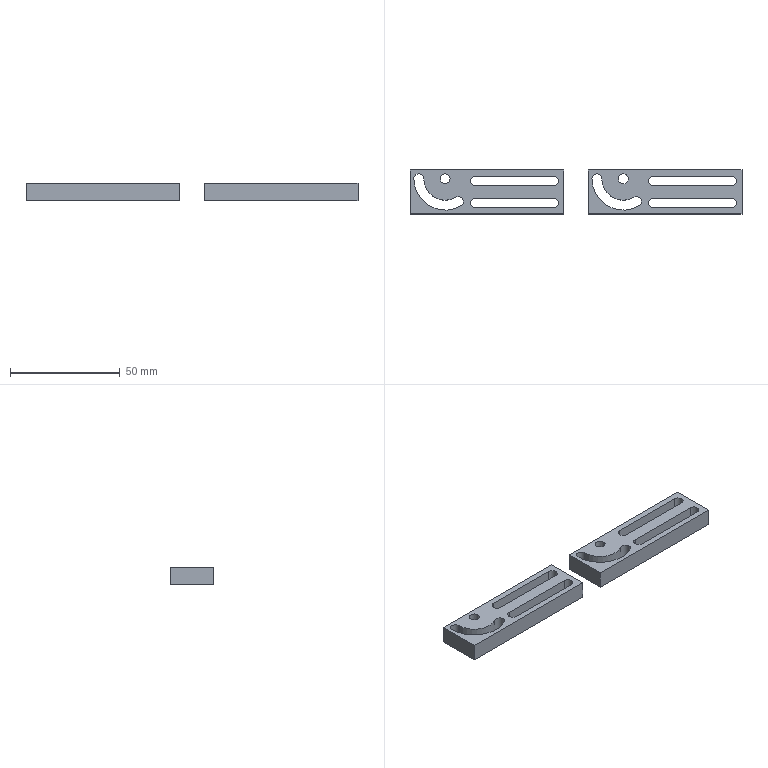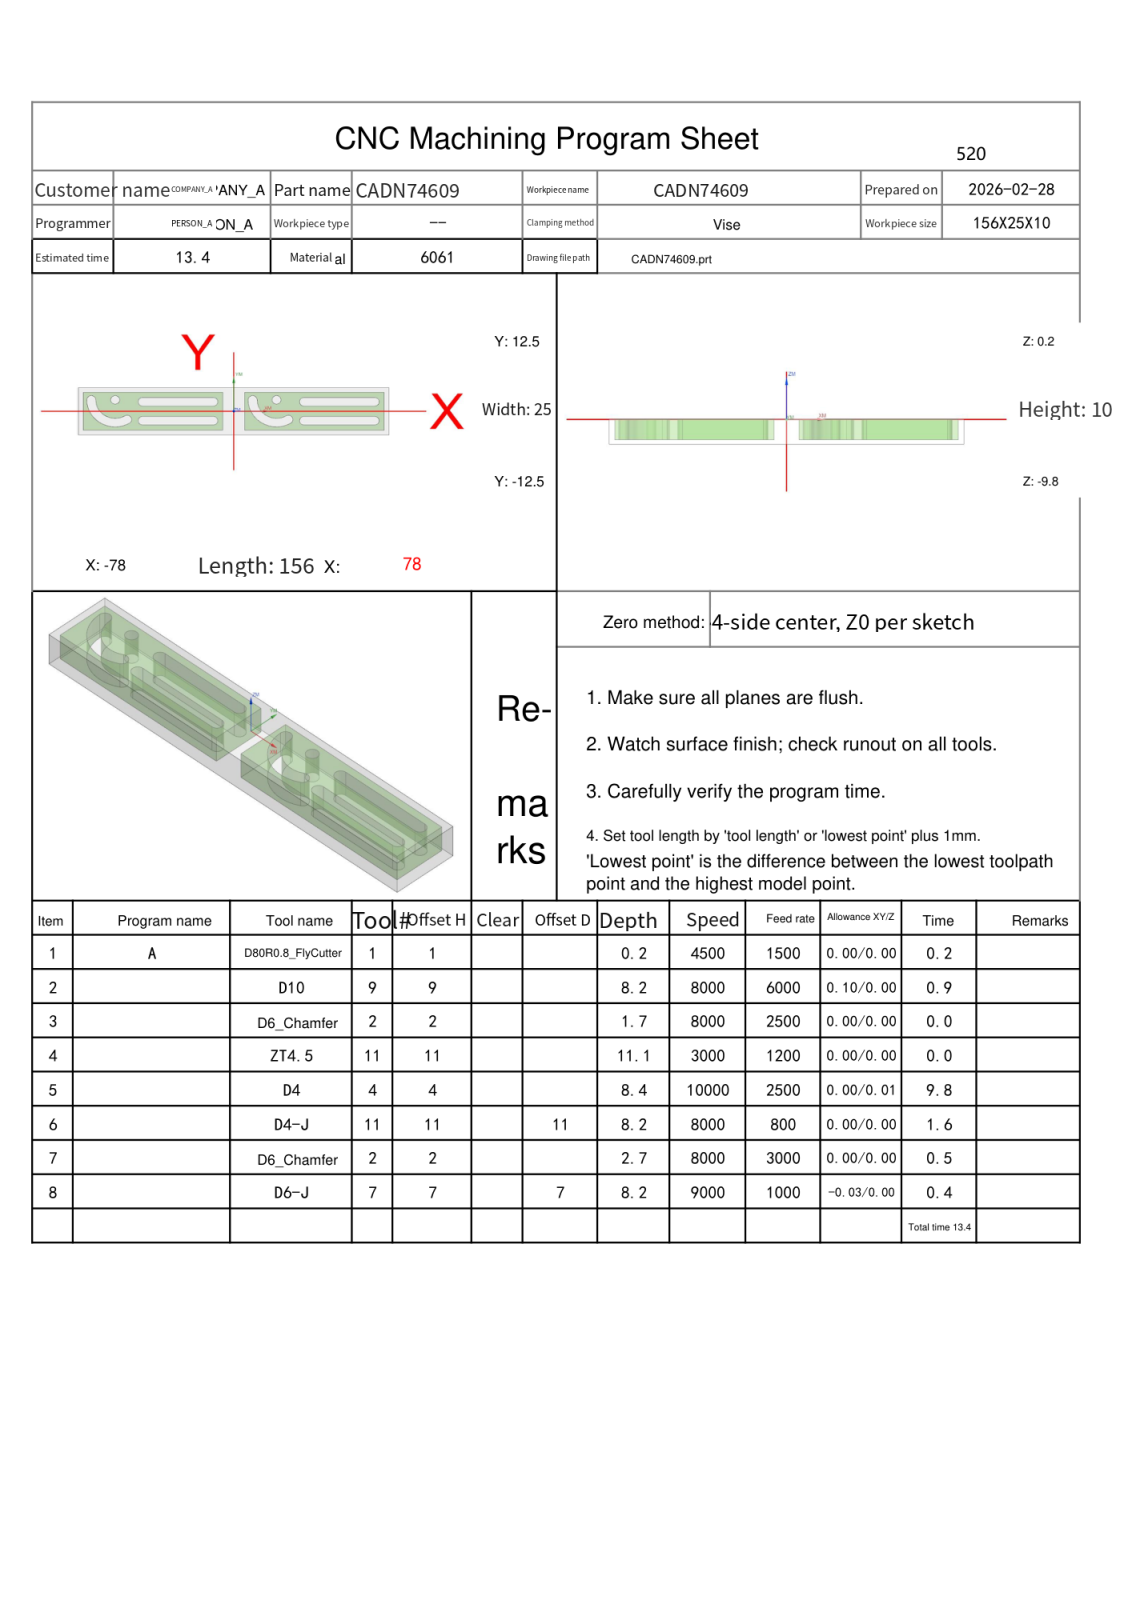NC program | NX | posted by the shop | part box 151 x 20 x 8 mm
Lines 1 to 275 of 3746:
%
O0001
(Machine time: 14.93 MIN)
(===Total Tool:6===)
(T1=D80R0.8-FlyCutter D=80.  R=0.8  D-  H01 Z=0.    )
(T9=D10     D=10.  R=0.   D-  H09 Z=-8.   )
(T2=D6_Chamfer   D=6.   R=0.   D-  H02 Z=-2.55 )
(T11=ZT4.5  D=4.5  DR_a=118 D-  H11 Z=-10.85)
(T4=D4      D=4.   R=0.   D-  H04 Z=-8.2  )
(T7=D6-J    D=6.   R=0.   D7  H07 Z=-8.   )
G80 G90 G17 G49 G40
G91 G28 Z0
M01
N1 T01 M06
(D80R0.8-FlyCutter  D=80. R=0.8 H=01 ce=0.00 di=0.00)
G00 G90 G54 X-120.5 Y0.0 M03 S4500
G43 H01 Z50.
M08
Z2.
G01 Z0.0 F1500.
X-115.5
X115.5
X120.5
Z2.
G00 Z50.
G91 G28 Z0.0
M05
M09
G91 G28 Z0.0
M01
N2 T09 M06
(D10  D=10. R=0. H=09 ce=0.10 di=0.00)
G00 G90 G54 X-40.5 Y-15.1 M03 S8000
G43 H09 Z50.
M08
Z.5
G01 X-75.5 Z.372 F6000.
G02 X-80.6 Y-10. Z.343 I0.0 J5.1
G01 Y10. Z.27
G02 X-75.5 Y15.1 Z.241 I5.1 J0.0
G01 X-5.5 Z-.014
G02 X-.4 Y10. Z-.043 I0.0 J-5.1
G01 Y-10. Z-.116
G02 X-5.5 Y-15.1 Z-.145 I-5.1 J0.0
G01 X-75.5 Z-.4
G02 X-80.6 Y-10. Z-.429 I0.0 J5.1
G01 Y10. Z-.502
G02 X-75.5 Y15.1 Z-.532 I5.1 J0.0
G01 X-5.5 Z-.787
G02 X-.4 Y10. Z-.816 I0.0 J-5.1
G01 Y-10. Z-.889
G02 X-5.5 Y-15.1 Z-.918 I-5.1 J0.0
G01 X-75.5 Z-1.173
G02 X-80.6 Y-10. Z-1.202 I0.0 J5.1
G01 Y10. Z-1.275
G02 X-75.5 Y15.1 Z-1.304 I5.1 J0.0
G01 X-5.5 Z-1.559
G02 X-.4 Y10. Z-1.589 I0.0 J-5.1
G01 Y-10. Z-1.661
G02 X-5.5 Y-15.1 Z-1.691 I-5.1 J0.0
G01 X-75.5 Z-1.946
G02 X-80.6 Y-10. Z-1.975 I0.0 J5.1
G01 Y10. Z-2.048
G02 X-75.5 Y15.1 Z-2.077 I5.1 J0.0
G01 X-5.5 Z-2.332
G02 X-.4 Y10. Z-2.361 I0.0 J-5.1
G01 Y-10. Z-2.434
G02 X-5.5 Y-15.1 Z-2.463 I-5.1 J0.0
G01 X-75.5 Z-2.718
G02 X-80.6 Y-10. Z-2.748 I0.0 J5.1
G01 Y10. Z-2.821
G02 X-75.5 Y15.1 Z-2.85 I5.1 J0.0
G01 X-5.5 Z-3.105
G02 X-.4 Y10. Z-3.134 I0.0 J-5.1
G01 Y-10. Z-3.207
G02 X-5.5 Y-15.1 Z-3.236 I-5.1 J0.0
G01 X-75.5 Z-3.491
G02 X-80.6 Y-10. Z-3.52 I0.0 J5.1
G01 Y10. Z-3.593
G02 X-75.5 Y15.1 Z-3.622 I5.1 J0.0
G01 X-5.5 Z-3.878
G02 X-.4 Y10. Z-3.907 I0.0 J-5.1
G01 Y-10. Z-3.98
G02 X-5.5 Y-15.1 Z-4.009 I-5.1 J0.0
G01 X-75.5 Z-4.264
G02 X-80.6 Y-10. Z-4.293 I0.0 J5.1
G01 Y10. Z-4.366
G02 X-75.5 Y15.1 Z-4.395 I5.1 J0.0
G01 X-5.5 Z-4.65
G02 X-.4 Y10. Z-4.679 I0.0 J-5.1
G01 Y-10. Z-4.752
G02 X-5.5 Y-15.1 Z-4.782 I-5.1 J0.0
G01 X-75.5 Z-5.037
G02 X-80.6 Y-10. Z-5.066 I0.0 J5.1
G01 Y10. Z-5.139
G02 X-75.5 Y15.1 Z-5.168 I5.1 J0.0
G01 X-5.5 Z-5.423
G02 X-.4 Y10. Z-5.452 I0.0 J-5.1
G01 Y-10. Z-5.525
G02 X-5.5 Y-15.1 Z-5.554 I-5.1 J0.0
G01 X-75.5 Z-5.809
G02 X-80.6 Y-10. Z-5.839 I0.0 J5.1
G01 Y10. Z-5.911
G02 X-75.5 Y15.1 Z-5.941 I5.1 J0.0
G01 X-5.5 Z-6.196
G02 X-.4 Y10. Z-6.225 I0.0 J-5.1
G01 Y-10. Z-6.298
G02 X-5.5 Y-15.1 Z-6.327 I-5.1 J0.0
G01 X-75.5 Z-6.582
G02 X-80.6 Y-10. Z-6.611 I0.0 J5.1
G01 Y10. Z-6.684
G02 X-75.5 Y15.1 Z-6.713 I5.1 J0.0
G01 X-5.5 Z-6.968
G02 X-.4 Y10. Z-6.998 I0.0 J-5.1
G01 Y-10. Z-7.071
G02 X-5.5 Y-15.1 Z-7.1 I-5.1 J0.0
G01 X-75.5 Z-7.355
G02 X-80.6 Y-10. Z-7.384 I0.0 J5.1
G01 Y10. Z-7.457
G02 X-75.5 Y15.1 Z-7.486 I5.1 J0.0
G01 X-5.5 Z-7.741
G02 X-.4 Y10. Z-7.77 I0.0 J-5.1
G01 Y-10. Z-7.843
G02 X-5.5 Y-15.1 Z-7.872 I-5.1 J0.0
G01 X-40.5 Z-8.
X-75.5
G02 X-80.6 Y-10. I0.0 J5.1
G01 Y10.
G02 X-75.5 Y15.1 I5.1 J0.0
G01 X-5.5
G02 X-.4 Y10. I0.0 J-5.1
G01 Y-10.
G02 X-5.5 Y-15.1 I-5.1 J0.0
G01 X-40.5
X-41.
Z-7.
G00 Z50.
X40.5
Z.5
G01 X5.5 Z.372
G02 X.4 Y-10. Z.343 I0.0 J5.1
G01 Y10. Z.27
G02 X5.5 Y15.1 Z.241 I5.1 J0.0
G01 X75.5 Z-.014
G02 X80.6 Y10. Z-.043 I0.0 J-5.1
G01 Y-10. Z-.116
G02 X75.5 Y-15.1 Z-.145 I-5.1 J0.0
G01 X5.5 Z-.4
G02 X.4 Y-10. Z-.429 I0.0 J5.1
G01 Y10. Z-.502
G02 X5.5 Y15.1 Z-.532 I5.1 J0.0
G01 X75.5 Z-.787
G02 X80.6 Y10. Z-.816 I0.0 J-5.1
G01 Y-10. Z-.889
G02 X75.5 Y-15.1 Z-.918 I-5.1 J0.0
G01 X5.5 Z-1.173
G02 X.4 Y-10. Z-1.202 I0.0 J5.1
G01 Y10. Z-1.275
G02 X5.5 Y15.1 Z-1.304 I5.1 J0.0
G01 X75.5 Z-1.559
G02 X80.6 Y10. Z-1.589 I0.0 J-5.1
G01 Y-10. Z-1.661
G02 X75.5 Y-15.1 Z-1.691 I-5.1 J0.0
G01 X5.5 Z-1.946
G02 X.4 Y-10. Z-1.975 I0.0 J5.1
G01 Y10. Z-2.048
G02 X5.5 Y15.1 Z-2.077 I5.1 J0.0
G01 X75.5 Z-2.332
G02 X80.6 Y10. Z-2.361 I0.0 J-5.1
G01 Y-10. Z-2.434
G02 X75.5 Y-15.1 Z-2.463 I-5.1 J0.0
G01 X5.5 Z-2.718
G02 X.4 Y-10. Z-2.748 I0.0 J5.1
G01 Y10. Z-2.821
G02 X5.5 Y15.1 Z-2.85 I5.1 J0.0
G01 X75.5 Z-3.105
G02 X80.6 Y10. Z-3.134 I0.0 J-5.1
G01 Y-10. Z-3.207
G02 X75.5 Y-15.1 Z-3.236 I-5.1 J0.0
G01 X5.5 Z-3.491
G02 X.4 Y-10. Z-3.52 I0.0 J5.1
G01 Y10. Z-3.593
G02 X5.5 Y15.1 Z-3.622 I5.1 J0.0
G01 X75.5 Z-3.878
G02 X80.6 Y10. Z-3.907 I0.0 J-5.1
G01 Y-10. Z-3.98
G02 X75.5 Y-15.1 Z-4.009 I-5.1 J0.0
G01 X5.5 Z-4.264
G02 X.4 Y-10. Z-4.293 I0.0 J5.1
G01 Y10. Z-4.366
G02 X5.5 Y15.1 Z-4.395 I5.1 J0.0
G01 X75.5 Z-4.65
G02 X80.6 Y10. Z-4.679 I0.0 J-5.1
G01 Y-10. Z-4.752
G02 X75.5 Y-15.1 Z-4.782 I-5.1 J0.0
G01 X5.5 Z-5.037
G02 X.4 Y-10. Z-5.066 I0.0 J5.1
G01 Y10. Z-5.139
G02 X5.5 Y15.1 Z-5.168 I5.1 J0.0
G01 X75.5 Z-5.423
G02 X80.6 Y10. Z-5.452 I0.0 J-5.1
G01 Y-10. Z-5.525
G02 X75.5 Y-15.1 Z-5.554 I-5.1 J0.0
G01 X5.5 Z-5.809
G02 X.4 Y-10. Z-5.839 I0.0 J5.1
G01 Y10. Z-5.911
G02 X5.5 Y15.1 Z-5.941 I5.1 J0.0
G01 X75.5 Z-6.196
G02 X80.6 Y10. Z-6.225 I0.0 J-5.1
G01 Y-10. Z-6.298
G02 X75.5 Y-15.1 Z-6.327 I-5.1 J0.0
G01 X5.5 Z-6.582
G02 X.4 Y-10. Z-6.611 I0.0 J5.1
G01 Y10. Z-6.684
G02 X5.5 Y15.1 Z-6.713 I5.1 J0.0
G01 X75.5 Z-6.968
G02 X80.6 Y10. Z-6.998 I0.0 J-5.1
G01 Y-10. Z-7.071
G02 X75.5 Y-15.1 Z-7.1 I-5.1 J0.0
G01 X5.5 Z-7.355
G02 X.4 Y-10. Z-7.384 I0.0 J5.1
G01 Y10. Z-7.457
G02 X5.5 Y15.1 Z-7.486 I5.1 J0.0
G01 X75.5 Z-7.741
G02 X80.6 Y10. Z-7.77 I0.0 J-5.1
G01 Y-10. Z-7.843
G02 X75.5 Y-15.1 Z-7.872 I-5.1 J0.0
G01 X40.5 Z-8.
X5.5
G02 X.4 Y-10. I0.0 J5.1
G01 Y10.
G02 X5.5 Y15.1 I5.1 J0.0
G01 X75.5
G02 X80.6 Y10. I0.0 J-5.1
G01 Y-10.
G02 X75.5 Y-15.1 I-5.1 J0.0
G01 X40.5
X40.
Z-7.
G00 Z50.
G91 G28 Z0.0
M05
M09
G91 G28 Z0.0
M01
N3 T02 M06
(D6_Chamfer  D=6. R=0. H=02 ce=0.00 di=0.00)
G00 G90 G54 X-59.5 Y6. M03 S8000
G43 H02 Z50.
M08
G98 G81 X-59.5 Y6. Z-1.5 R1. F2500.
X21.5
G80
G00 Z50.
G91 G28 Z0.0
M05
M09
G91 G28 Z0.0
M01
N4 T11 M06
(ZT4.5 D=4.5 DR_a=118 H=11)
G00 G90 G54 X-59.5 Y6. M03 S3000
G43 H11 Z50.
M08
G98 G83 X-59.5 Y6. Z-10.852 R1. F1200. Q1.5
X21.5
G80
G00 Z50.
G91 G28 Z0.0
M05
M09
G91 G28 Z0.0
M01